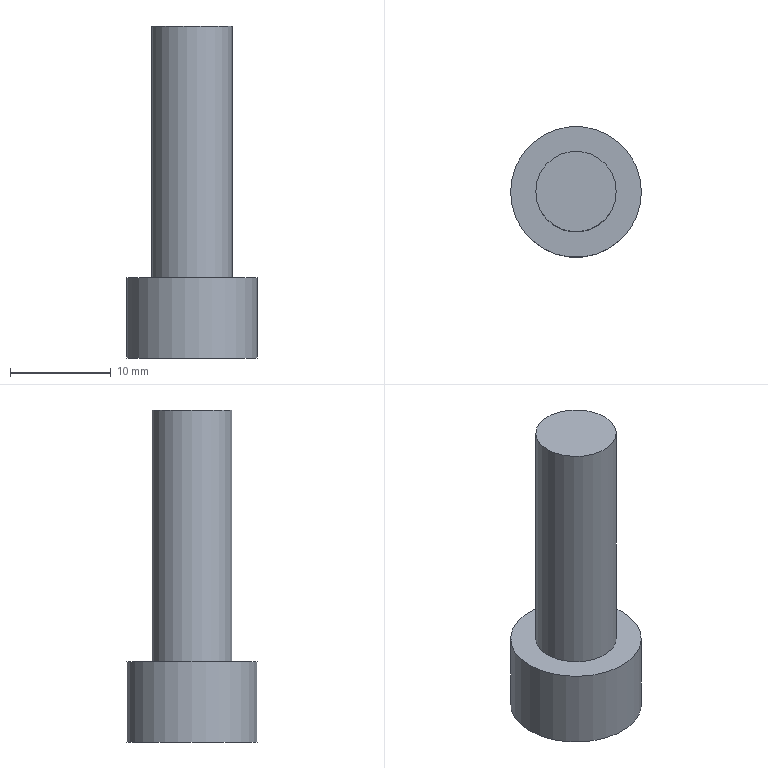Part | STEP file | 1 solid | 12 faces | box 13 x 13 x 33 mm | volume 2154 mm3 | plane 10 | cylinder 2 | commonest cylinder face diameters 8 x1 13 x1
STEP:
#1=CARTESIAN_POINT('',(0.,0.,0.));
#2=DIRECTION('',(0.,0.,1.));
#3=DIRECTION('',(1.,0.,0.));
#4=AXIS2_PLACEMENT_3D('',#1,#2,#3);
#5=CARTESIAN_POINT('',(1550.747,372.48,24.619));
#6=VERTEX_POINT('',#5);
#7=CARTESIAN_POINT('',(1557.247,372.48,24.619));
#8=DIRECTION('',(0.,0.,-1.));
#9=DIRECTION('',(-1.,0.,0.));
#10=AXIS2_PLACEMENT_3D('',#7,#8,#9);
#11=CIRCLE('',#10,6.5);
#12=CARTESIAN_POINT('',(1550.747,372.48,24.619));
#13=DIRECTION('',(0.,0.,1.));
#14=DIRECTION('',(1.,0.,0.));
#15=AXIS2_PLACEMENT_3D('',#12,#13,#14);
#16=PLANE('',#15);
#17=CARTESIAN_POINT('',(0.,0.));
#18=CARTESIAN_POINT('',(0.,11.258));
#19=CARTESIAN_POINT('',(9.75,5.629));
#20=CARTESIAN_POINT('',(19.5,0.));
#21=CARTESIAN_POINT('',(9.75,-5.629));
#22=CARTESIAN_POINT('',(0.,-11.258));
#23=CARTESIAN_POINT('',(0.,0.));
#24=(BOUNDED_CURVE()B_SPLINE_CURVE(2,(#17,#18,#19,#20,#21,#22,#23),.UNSPECIFIED.,.T.,.F.)B_SPLINE_CURVE_WITH_KNOTS((1,2,2,2,2,1),(-2.094,0.,2.094,4.189,6.283,8.378),.UNSPECIFIED.)CURVE()GEOMETRIC_REPRESENTATION_ITEM()RATIONAL_B_SPLINE_CURVE((1.,0.5,1.,0.5,1.,0.5,1.))REPRESENTATION_ITEM(''));
#25=(GEOMETRIC_REPRESENTATION_CONTEXT(2)PARAMETRIC_REPRESENTATION_CONTEXT()REPRESENTATION_CONTEXT('',''));
#26=DEFINITIONAL_REPRESENTATION('',(#24),#25);
#27=PCURVE('',#16,#26);
#28=CARTESIAN_POINT('',(1557.247,372.48,79.519));
#29=DIRECTION('',(0.,0.,-1.));
#30=DIRECTION('',(-1.,0.,0.));
#31=AXIS2_PLACEMENT_3D('',#28,#29,#30);
#32=CYLINDRICAL_SURFACE('',#31,6.5);
#33=CARTESIAN_POINT('',(0.,54.9));
#34=DIRECTION('',(1.,0.));
#35=VECTOR('',#34,1.);
#36=LINE('',#33,#35);
#37=(GEOMETRIC_REPRESENTATION_CONTEXT(2)PARAMETRIC_REPRESENTATION_CONTEXT()REPRESENTATION_CONTEXT('',''));
#38=DEFINITIONAL_REPRESENTATION('',(#36),#37);
#39=PCURVE('',#32,#38);
#40=SURFACE_CURVE('',#11,(#27,#39),.PCURVE_S1.);
#41=EDGE_CURVE('',#6,#6,#40,.T.);
#42=ORIENTED_EDGE('',*,*,#41,.T.);
#43=EDGE_LOOP('',(#42));
#44=FACE_BOUND('',#43,.T.);
#45=CARTESIAN_POINT('',(1558.979,375.48,24.619));
#46=VERTEX_POINT('',#45);
#47=CARTESIAN_POINT('',(1555.515,375.48,24.619));
#48=VERTEX_POINT('',#47);
#49=CARTESIAN_POINT('',(1558.979,375.48,24.619));
#50=DIRECTION('',(-1.,0.,0.));
#51=VECTOR('',#50,1.);
#52=LINE('',#49,#51);
#53=CARTESIAN_POINT('',(8.232,3.));
#54=DIRECTION('',(-1.,0.));
#55=VECTOR('',#54,1.);
#56=LINE('',#53,#55);
#57=(GEOMETRIC_REPRESENTATION_CONTEXT(2)PARAMETRIC_REPRESENTATION_CONTEXT()REPRESENTATION_CONTEXT('',''));
#58=DEFINITIONAL_REPRESENTATION('',(#56),#57);
#59=PCURVE('',#16,#58);
#60=CARTESIAN_POINT('',(1558.979,375.48,29.899));
#61=DIRECTION('',(0.,-1.,0.));
#62=DIRECTION('',(-1.,0.,0.));
#63=AXIS2_PLACEMENT_3D('',#60,#61,#62);
#64=PLANE('',#63);
#65=CARTESIAN_POINT('',(0.,5.28));
#66=DIRECTION('',(1.,0.));
#67=VECTOR('',#66,1.);
#68=LINE('',#65,#67);
#69=(GEOMETRIC_REPRESENTATION_CONTEXT(2)PARAMETRIC_REPRESENTATION_CONTEXT()REPRESENTATION_CONTEXT('',''));
#70=DEFINITIONAL_REPRESENTATION('',(#68),#69);
#71=PCURVE('',#64,#70);
#72=SURFACE_CURVE('',#52,(#59,#71),.PCURVE_S1.);
#73=EDGE_CURVE('',#46,#48,#72,.T.);
#74=ORIENTED_EDGE('',*,*,#73,.T.);
#75=CARTESIAN_POINT('',(1553.783,372.48,24.619));
#76=VERTEX_POINT('',#75);
#77=CARTESIAN_POINT('',(1555.515,375.48,24.619));
#78=DIRECTION('',(-0.5,-0.866,0.));
#79=VECTOR('',#78,1.);
#80=LINE('',#77,#79);
#81=CARTESIAN_POINT('',(4.768,3.));
#82=DIRECTION('',(-0.5,-0.866));
#83=VECTOR('',#82,1.);
#84=LINE('',#81,#83);
#85=(GEOMETRIC_REPRESENTATION_CONTEXT(2)PARAMETRIC_REPRESENTATION_CONTEXT()REPRESENTATION_CONTEXT('',''));
#86=DEFINITIONAL_REPRESENTATION('',(#84),#85);
#87=PCURVE('',#16,#86);
#88=CARTESIAN_POINT('',(1555.515,375.48,29.899));
#89=DIRECTION('',(0.866,-0.5,0.));
#90=DIRECTION('',(-0.5,-0.866,0.));
#91=AXIS2_PLACEMENT_3D('',#88,#89,#90);
#92=PLANE('',#91);
#93=CARTESIAN_POINT('',(0.,5.28));
#94=DIRECTION('',(1.,0.));
#95=VECTOR('',#94,1.);
#96=LINE('',#93,#95);
#97=(GEOMETRIC_REPRESENTATION_CONTEXT(2)PARAMETRIC_REPRESENTATION_CONTEXT()REPRESENTATION_CONTEXT('',''));
#98=DEFINITIONAL_REPRESENTATION('',(#96),#97);
#99=PCURVE('',#92,#98);
#100=SURFACE_CURVE('',#80,(#87,#99),.PCURVE_S1.);
#101=EDGE_CURVE('',#48,#76,#100,.T.);
#102=ORIENTED_EDGE('',*,*,#101,.T.);
#103=CARTESIAN_POINT('',(1555.515,369.48,24.619));
#104=VERTEX_POINT('',#103);
#105=CARTESIAN_POINT('',(1553.783,372.48,24.619));
#106=DIRECTION('',(0.5,-0.866,0.));
#107=VECTOR('',#106,1.);
#108=LINE('',#105,#107);
#109=CARTESIAN_POINT('',(3.036,0.));
#110=DIRECTION('',(0.5,-0.866));
#111=VECTOR('',#110,1.);
#112=LINE('',#109,#111);
#113=(GEOMETRIC_REPRESENTATION_CONTEXT(2)PARAMETRIC_REPRESENTATION_CONTEXT()REPRESENTATION_CONTEXT('',''));
#114=DEFINITIONAL_REPRESENTATION('',(#112),#113);
#115=PCURVE('',#16,#114);
#116=CARTESIAN_POINT('',(1553.783,372.48,29.899));
#117=DIRECTION('',(0.866,0.5,0.));
#118=DIRECTION('',(0.5,-0.866,0.));
#119=AXIS2_PLACEMENT_3D('',#116,#117,#118);
#120=PLANE('',#119);
#121=CARTESIAN_POINT('',(0.,5.28));
#122=DIRECTION('',(1.,0.));
#123=VECTOR('',#122,1.);
#124=LINE('',#121,#123);
#125=(GEOMETRIC_REPRESENTATION_CONTEXT(2)PARAMETRIC_REPRESENTATION_CONTEXT()REPRESENTATION_CONTEXT('',''));
#126=DEFINITIONAL_REPRESENTATION('',(#124),#125);
#127=PCURVE('',#120,#126);
#128=SURFACE_CURVE('',#108,(#115,#127),.PCURVE_S1.);
#129=EDGE_CURVE('',#76,#104,#128,.T.);
#130=ORIENTED_EDGE('',*,*,#129,.T.);
#131=CARTESIAN_POINT('',(1558.979,369.48,24.619));
#132=VERTEX_POINT('',#131);
#133=CARTESIAN_POINT('',(1555.515,369.48,24.619));
#134=DIRECTION('',(1.,0.,0.));
#135=VECTOR('',#134,1.);
#136=LINE('',#133,#135);
#137=CARTESIAN_POINT('',(4.768,-3.));
#138=DIRECTION('',(1.,0.));
#139=VECTOR('',#138,1.);
#140=LINE('',#137,#139);
#141=(GEOMETRIC_REPRESENTATION_CONTEXT(2)PARAMETRIC_REPRESENTATION_CONTEXT()REPRESENTATION_CONTEXT('',''));
#142=DEFINITIONAL_REPRESENTATION('',(#140),#141);
#143=PCURVE('',#16,#142);
#144=CARTESIAN_POINT('',(1555.515,369.48,29.899));
#145=DIRECTION('',(0.,1.,0.));
#146=DIRECTION('',(1.,0.,0.));
#147=AXIS2_PLACEMENT_3D('',#144,#145,#146);
#148=PLANE('',#147);
#149=CARTESIAN_POINT('',(0.,5.28));
#150=DIRECTION('',(1.,0.));
#151=VECTOR('',#150,1.);
#152=LINE('',#149,#151);
#153=(GEOMETRIC_REPRESENTATION_CONTEXT(2)PARAMETRIC_REPRESENTATION_CONTEXT()REPRESENTATION_CONTEXT('',''));
#154=DEFINITIONAL_REPRESENTATION('',(#152),#153);
#155=PCURVE('',#148,#154);
#156=SURFACE_CURVE('',#136,(#143,#155),.PCURVE_S1.);
#157=EDGE_CURVE('',#104,#132,#156,.T.);
#158=ORIENTED_EDGE('',*,*,#157,.T.);
#159=CARTESIAN_POINT('',(1560.711,372.48,24.619));
#160=VERTEX_POINT('',#159);
#161=CARTESIAN_POINT('',(1558.979,369.48,24.619));
#162=DIRECTION('',(0.5,0.866,0.));
#163=VECTOR('',#162,1.);
#164=LINE('',#161,#163);
#165=CARTESIAN_POINT('',(8.232,-3.));
#166=DIRECTION('',(0.5,0.866));
#167=VECTOR('',#166,1.);
#168=LINE('',#165,#167);
#169=(GEOMETRIC_REPRESENTATION_CONTEXT(2)PARAMETRIC_REPRESENTATION_CONTEXT()REPRESENTATION_CONTEXT('',''));
#170=DEFINITIONAL_REPRESENTATION('',(#168),#169);
#171=PCURVE('',#16,#170);
#172=CARTESIAN_POINT('',(1558.979,369.48,29.899));
#173=DIRECTION('',(-0.866,0.5,0.));
#174=DIRECTION('',(0.5,0.866,0.));
#175=AXIS2_PLACEMENT_3D('',#172,#173,#174);
#176=PLANE('',#175);
#177=CARTESIAN_POINT('',(0.,5.28));
#178=DIRECTION('',(1.,0.));
#179=VECTOR('',#178,1.);
#180=LINE('',#177,#179);
#181=(GEOMETRIC_REPRESENTATION_CONTEXT(2)PARAMETRIC_REPRESENTATION_CONTEXT()REPRESENTATION_CONTEXT('',''));
#182=DEFINITIONAL_REPRESENTATION('',(#180),#181);
#183=PCURVE('',#176,#182);
#184=SURFACE_CURVE('',#164,(#171,#183),.PCURVE_S1.);
#185=EDGE_CURVE('',#132,#160,#184,.T.);
#186=ORIENTED_EDGE('',*,*,#185,.T.);
#187=CARTESIAN_POINT('',(1560.711,372.48,24.619));
#188=DIRECTION('',(-0.5,0.866,0.));
#189=VECTOR('',#188,1.);
#190=LINE('',#187,#189);
#191=CARTESIAN_POINT('',(9.964,0.));
#192=DIRECTION('',(-0.5,0.866));
#193=VECTOR('',#192,1.);
#194=LINE('',#191,#193);
#195=(GEOMETRIC_REPRESENTATION_CONTEXT(2)PARAMETRIC_REPRESENTATION_CONTEXT()REPRESENTATION_CONTEXT('',''));
#196=DEFINITIONAL_REPRESENTATION('',(#194),#195);
#197=PCURVE('',#16,#196);
#198=CARTESIAN_POINT('',(1560.711,372.48,29.899));
#199=DIRECTION('',(-0.866,-0.5,0.));
#200=DIRECTION('',(-0.5,0.866,0.));
#201=AXIS2_PLACEMENT_3D('',#198,#199,#200);
#202=PLANE('',#201);
#203=CARTESIAN_POINT('',(0.,5.28));
#204=DIRECTION('',(1.,0.));
#205=VECTOR('',#204,1.);
#206=LINE('',#203,#205);
#207=(GEOMETRIC_REPRESENTATION_CONTEXT(2)PARAMETRIC_REPRESENTATION_CONTEXT()REPRESENTATION_CONTEXT('',''));
#208=DEFINITIONAL_REPRESENTATION('',(#206),#207);
#209=PCURVE('',#202,#208);
#210=SURFACE_CURVE('',#190,(#197,#209),.PCURVE_S1.);
#211=EDGE_CURVE('',#160,#46,#210,.T.);
#212=ORIENTED_EDGE('',*,*,#211,.T.);
#213=EDGE_LOOP('',(#74,#102,#130,#158,#186,#212));
#214=FACE_BOUND('',#213,.T.);
#215=ADVANCED_FACE('',(#44,#214),#16,.F.);
#216=ORIENTED_EDGE('',*,*,#41,.F.);
#217=CARTESIAN_POINT('',(1550.747,372.48,32.619));
#218=VERTEX_POINT('',#217);
#219=CARTESIAN_POINT('',(1550.747,372.48,32.619));
#220=CARTESIAN_POINT('',(1550.747,372.48,24.619));
#221=B_SPLINE_CURVE_WITH_KNOTS('',1,(#219,#220),.UNSPECIFIED.,.F.,.F.,(2,2),(46.9,54.9),.PIECEWISE_BEZIER_KNOTS.);
#222=CARTESIAN_POINT('',(0.,0.));
#223=DIRECTION('',(0.,1.));
#224=VECTOR('',#223,1.);
#225=LINE('',#222,#224);
#226=(GEOMETRIC_REPRESENTATION_CONTEXT(2)PARAMETRIC_REPRESENTATION_CONTEXT()REPRESENTATION_CONTEXT('',''));
#227=DEFINITIONAL_REPRESENTATION('',(#225),#226);
#228=PCURVE('',#32,#227);
#229=CARTESIAN_POINT('',(6.283,0.));
#230=DIRECTION('',(0.,1.));
#231=VECTOR('',#230,1.);
#232=LINE('',#229,#231);
#233=(GEOMETRIC_REPRESENTATION_CONTEXT(2)PARAMETRIC_REPRESENTATION_CONTEXT()REPRESENTATION_CONTEXT('',''));
#234=DEFINITIONAL_REPRESENTATION('',(#232),#233);
#235=PCURVE('',#32,#234);
#236=SEAM_CURVE('',#221,(#228,#235),.PCURVE_S1.);
#237=EDGE_CURVE('',#218,#6,#236,.T.);
#238=ORIENTED_EDGE('',*,*,#237,.F.);
#239=CARTESIAN_POINT('',(1557.247,372.48,32.619));
#240=DIRECTION('',(0.,0.,-1.));
#241=DIRECTION('',(-1.,0.,0.));
#242=AXIS2_PLACEMENT_3D('',#239,#240,#241);
#243=CIRCLE('',#242,6.5);
#244=CARTESIAN_POINT('',(0.,46.9));
#245=DIRECTION('',(1.,0.));
#246=VECTOR('',#245,1.);
#247=LINE('',#244,#246);
#248=(GEOMETRIC_REPRESENTATION_CONTEXT(2)PARAMETRIC_REPRESENTATION_CONTEXT()REPRESENTATION_CONTEXT('',''));
#249=DEFINITIONAL_REPRESENTATION('',(#247),#248);
#250=PCURVE('',#32,#249);
#251=CARTESIAN_POINT('',(1553.247,372.48,32.619));
#252=DIRECTION('',(0.,0.,-1.));
#253=DIRECTION('',(-1.,0.,0.));
#254=AXIS2_PLACEMENT_3D('',#251,#252,#253);
#255=PLANE('',#254);
#256=CARTESIAN_POINT('',(-4.,0.));
#257=DIRECTION('',(1.,0.));
#258=AXIS2_PLACEMENT_2D('',#256,#257);
#259=CIRCLE('',#258,6.5);
#260=(GEOMETRIC_REPRESENTATION_CONTEXT(2)PARAMETRIC_REPRESENTATION_CONTEXT()REPRESENTATION_CONTEXT('',''));
#261=DEFINITIONAL_REPRESENTATION('',(#259),#260);
#262=PCURVE('',#255,#261);
#263=SURFACE_CURVE('',#243,(#250,#262),.PCURVE_S1.);
#264=EDGE_CURVE('',#218,#218,#263,.T.);
#265=ORIENTED_EDGE('',*,*,#264,.T.);
#266=ORIENTED_EDGE('',*,*,#237,.T.);
#267=EDGE_LOOP('',(#216,#238,#265,#266));
#268=FACE_BOUND('',#267,.T.);
#269=ADVANCED_FACE('',(#268),#32,.T.);
#270=ORIENTED_EDGE('',*,*,#264,.F.);
#271=EDGE_LOOP('',(#270));
#272=FACE_BOUND('',#271,.T.);
#273=CARTESIAN_POINT('',(1553.247,372.48,32.619));
#274=VERTEX_POINT('',#273);
#275=CARTESIAN_POINT('',(1557.247,372.48,32.619));
#276=DIRECTION('',(0.,0.,-1.));
#277=DIRECTION('',(-1.,0.,0.));
#278=AXIS2_PLACEMENT_3D('',#275,#276,#277);
#279=CIRCLE('',#278,4.);
#280=CARTESIAN_POINT('',(-4.,0.));
#281=DIRECTION('',(1.,0.));
#282=AXIS2_PLACEMENT_2D('',#280,#281);
#283=CIRCLE('',#282,4.);
#284=(GEOMETRIC_REPRESENTATION_CONTEXT(2)PARAMETRIC_REPRESENTATION_CONTEXT()REPRESENTATION_CONTEXT('',''));
#285=DEFINITIONAL_REPRESENTATION('',(#283),#284);
#286=PCURVE('',#255,#285);
#287=CARTESIAN_POINT('',(1557.247,372.48,79.519));
#288=DIRECTION('',(0.,0.,-1.));
#289=DIRECTION('',(-1.,0.,0.));
#290=AXIS2_PLACEMENT_3D('',#287,#288,#289);
#291=CYLINDRICAL_SURFACE('',#290,4.);
#292=CARTESIAN_POINT('',(0.,46.9));
#293=DIRECTION('',(1.,0.));
#294=VECTOR('',#293,1.);
#295=LINE('',#292,#294);
#296=(GEOMETRIC_REPRESENTATION_CONTEXT(2)PARAMETRIC_REPRESENTATION_CONTEXT()REPRESENTATION_CONTEXT('',''));
#297=DEFINITIONAL_REPRESENTATION('',(#295),#296);
#298=PCURVE('',#291,#297);
#299=SURFACE_CURVE('',#279,(#286,#298),.PCURVE_S1.);
#300=EDGE_CURVE('',#274,#274,#299,.T.);
#301=ORIENTED_EDGE('',*,*,#300,.T.);
#302=EDGE_LOOP('',(#301));
#303=FACE_BOUND('',#302,.T.);
#304=ADVANCED_FACE('',(#272,#303),#255,.F.);
#305=ORIENTED_EDGE('',*,*,#300,.F.);
#306=CARTESIAN_POINT('',(1553.247,372.48,57.619));
#307=VERTEX_POINT('',#306);
#308=CARTESIAN_POINT('',(1553.247,372.48,57.619));
#309=CARTESIAN_POINT('',(1553.247,372.48,32.619));
#310=B_SPLINE_CURVE_WITH_KNOTS('',1,(#308,#309),.UNSPECIFIED.,.F.,.F.,(2,2),(21.9,46.9),.PIECEWISE_BEZIER_KNOTS.);
#311=CARTESIAN_POINT('',(0.,0.));
#312=DIRECTION('',(0.,1.));
#313=VECTOR('',#312,1.);
#314=LINE('',#311,#313);
#315=(GEOMETRIC_REPRESENTATION_CONTEXT(2)PARAMETRIC_REPRESENTATION_CONTEXT()REPRESENTATION_CONTEXT('',''));
#316=DEFINITIONAL_REPRESENTATION('',(#314),#315);
#317=PCURVE('',#291,#316);
#318=CARTESIAN_POINT('',(6.283,0.));
#319=DIRECTION('',(0.,1.));
#320=VECTOR('',#319,1.);
#321=LINE('',#318,#320);
#322=(GEOMETRIC_REPRESENTATION_CONTEXT(2)PARAMETRIC_REPRESENTATION_CONTEXT()REPRESENTATION_CONTEXT('',''));
#323=DEFINITIONAL_REPRESENTATION('',(#321),#322);
#324=PCURVE('',#291,#323);
#325=SEAM_CURVE('',#310,(#317,#324),.PCURVE_S1.);
#326=EDGE_CURVE('',#307,#274,#325,.T.);
#327=ORIENTED_EDGE('',*,*,#326,.F.);
#328=CARTESIAN_POINT('',(1557.247,372.48,57.619));
#329=DIRECTION('',(0.,0.,-1.));
#330=DIRECTION('',(-1.,0.,0.));
#331=AXIS2_PLACEMENT_3D('',#328,#329,#330);
#332=CIRCLE('',#331,4.);
#333=CARTESIAN_POINT('',(0.,21.9));
#334=DIRECTION('',(1.,0.));
#335=VECTOR('',#334,1.);
#336=LINE('',#333,#335);
#337=(GEOMETRIC_REPRESENTATION_CONTEXT(2)PARAMETRIC_REPRESENTATION_CONTEXT()REPRESENTATION_CONTEXT('',''));
#338=DEFINITIONAL_REPRESENTATION('',(#336),#337);
#339=PCURVE('',#291,#338);
#340=CARTESIAN_POINT('',(1557.247,372.48,57.619));
#341=DIRECTION('',(0.,0.,-1.));
#342=DIRECTION('',(-1.,0.,0.));
#343=AXIS2_PLACEMENT_3D('',#340,#341,#342);
#344=PLANE('',#343);
#345=CARTESIAN_POINT('',(0.,0.));
#346=DIRECTION('',(1.,0.));
#347=AXIS2_PLACEMENT_2D('',#345,#346);
#348=CIRCLE('',#347,4.);
#349=(GEOMETRIC_REPRESENTATION_CONTEXT(2)PARAMETRIC_REPRESENTATION_CONTEXT()REPRESENTATION_CONTEXT('',''));
#350=DEFINITIONAL_REPRESENTATION('',(#348),#349);
#351=PCURVE('',#344,#350);
#352=SURFACE_CURVE('',#332,(#339,#351),.PCURVE_S1.);
#353=EDGE_CURVE('',#307,#307,#352,.T.);
#354=ORIENTED_EDGE('',*,*,#353,.T.);
#355=ORIENTED_EDGE('',*,*,#326,.T.);
#356=EDGE_LOOP('',(#305,#327,#354,#355));
#357=FACE_BOUND('',#356,.T.);
#358=ADVANCED_FACE('',(#357),#291,.T.);
#359=ORIENTED_EDGE('',*,*,#353,.F.);
#360=EDGE_LOOP('',(#359));
#361=FACE_BOUND('',#360,.T.);
#362=ADVANCED_FACE('',(#361),#344,.F.);
#363=ORIENTED_EDGE('',*,*,#73,.F.);
#364=CARTESIAN_POINT('',(1558.979,375.48,29.899));
#365=VERTEX_POINT('',#364);
#366=CARTESIAN_POINT('',(1558.979,375.48,29.899));
#367=DIRECTION('',(0.,0.,1.));
#368=VECTOR('',#367,1.);
#369=LINE('',#366,#368);
#370=CARTESIAN_POINT('',(0.,0.));
#371=DIRECTION('',(0.,-1.));
#372=VECTOR('',#371,1.);
#373=LINE('',#370,#372);
#374=(GEOMETRIC_REPRESENTATION_CONTEXT(2)PARAMETRIC_REPRESENTATION_CONTEXT()REPRESENTATION_CONTEXT('',''));
#375=DEFINITIONAL_REPRESENTATION('',(#373),#374);
#376=PCURVE('',#64,#375);
#377=CARTESIAN_POINT('',(3.464,0.));
#378=DIRECTION('',(0.,-1.));
#379=VECTOR('',#378,1.);
#380=LINE('',#377,#379);
#381=(GEOMETRIC_REPRESENTATION_CONTEXT(2)PARAMETRIC_REPRESENTATION_CONTEXT()REPRESENTATION_CONTEXT('',''));
#382=DEFINITIONAL_REPRESENTATION('',(#380),#381);
#383=PCURVE('',#202,#382);
#384=SURFACE_CURVE('',#369,(#376,#383),.PCURVE_S1.);
#385=EDGE_CURVE('',#46,#365,#384,.T.);
#386=ORIENTED_EDGE('',*,*,#385,.T.);
#387=CARTESIAN_POINT('',(1555.515,375.48,29.899));
#388=VERTEX_POINT('',#387);
#389=CARTESIAN_POINT('',(1558.979,375.48,29.899));
#390=DIRECTION('',(1.,0.,0.));
#391=VECTOR('',#390,1.);
#392=LINE('',#389,#391);
#393=CARTESIAN_POINT('',(0.,0.));
#394=DIRECTION('',(-1.,0.));
#395=VECTOR('',#394,1.);
#396=LINE('',#393,#395);
#397=(GEOMETRIC_REPRESENTATION_CONTEXT(2)PARAMETRIC_REPRESENTATION_CONTEXT()REPRESENTATION_CONTEXT('',''));
#398=DEFINITIONAL_REPRESENTATION('',(#396),#397);
#399=PCURVE('',#64,#398);
#400=CARTESIAN_POINT('',(1557.247,372.48,29.899));
#401=DIRECTION('',(0.,0.,1.));
#402=DIRECTION('',(1.,0.,0.));
#403=AXIS2_PLACEMENT_3D('',#400,#401,#402);
#404=PLANE('',#403);
#405=CARTESIAN_POINT('',(1.732,3.));
#406=DIRECTION('',(1.,0.));
#407=VECTOR('',#406,1.);
#408=LINE('',#405,#407);
#409=(GEOMETRIC_REPRESENTATION_CONTEXT(2)PARAMETRIC_REPRESENTATION_CONTEXT()REPRESENTATION_CONTEXT('',''));
#410=DEFINITIONAL_REPRESENTATION('',(#408),#409);
#411=PCURVE('',#404,#410);
#412=SURFACE_CURVE('',#392,(#399,#411),.PCURVE_S1.);
#413=EDGE_CURVE('',#388,#365,#412,.T.);
#414=ORIENTED_EDGE('',*,*,#413,.F.);
#415=CARTESIAN_POINT('',(1555.515,375.48,29.899));
#416=DIRECTION('',(0.,0.,1.));
#417=VECTOR('',#416,1.);
#418=LINE('',#415,#417);
#419=CARTESIAN_POINT('',(3.464,0.));
#420=DIRECTION('',(0.,-1.));
#421=VECTOR('',#420,1.);
#422=LINE('',#419,#421);
#423=(GEOMETRIC_REPRESENTATION_CONTEXT(2)PARAMETRIC_REPRESENTATION_CONTEXT()REPRESENTATION_CONTEXT('',''));
#424=DEFINITIONAL_REPRESENTATION('',(#422),#423);
#425=PCURVE('',#64,#424);
#426=CARTESIAN_POINT('',(0.,0.));
#427=DIRECTION('',(0.,-1.));
#428=VECTOR('',#427,1.);
#429=LINE('',#426,#428);
#430=(GEOMETRIC_REPRESENTATION_CONTEXT(2)PARAMETRIC_REPRESENTATION_CONTEXT()REPRESENTATION_CONTEXT('',''));
#431=DEFINITIONAL_REPRESENTATION('',(#429),#430);
#432=PCURVE('',#92,#431);
#433=SURFACE_CURVE('',#418,(#425,#432),.PCURVE_S1.);
#434=EDGE_CURVE('',#48,#388,#433,.T.);
#435=ORIENTED_EDGE('',*,*,#434,.F.);
#436=EDGE_LOOP('',(#363,#386,#414,#435));
#437=FACE_BOUND('',#436,.T.);
#438=ADVANCED_FACE('',(#437),#64,.T.);
#439=ORIENTED_EDGE('',*,*,#101,.F.);
#440=ORIENTED_EDGE('',*,*,#434,.T.);
#441=CARTESIAN_POINT('',(1553.783,372.48,29.899));
#442=VERTEX_POINT('',#441);
#443=CARTESIAN_POINT('',(1555.515,375.48,29.899));
#444=DIRECTION('',(0.5,0.866,0.));
#445=VECTOR('',#444,1.);
#446=LINE('',#443,#445);
#447=CARTESIAN_POINT('',(0.,0.));
#448=DIRECTION('',(-1.,0.));
#449=VECTOR('',#448,1.);
#450=LINE('',#447,#449);
#451=(GEOMETRIC_REPRESENTATION_CONTEXT(2)PARAMETRIC_REPRESENTATION_CONTEXT()REPRESENTATION_CONTEXT('',''));
#452=DEFINITIONAL_REPRESENTATION('',(#450),#451);
#453=PCURVE('',#92,#452);
#454=CARTESIAN_POINT('',(-1.732,3.));
#455=DIRECTION('',(0.5,0.866));
#456=VECTOR('',#455,1.);
#457=LINE('',#454,#456);
#458=(GEOMETRIC_REPRESENTATION_CONTEXT(2)PARAMETRIC_REPRESENTATION_CONTEXT()REPRESENTATION_CONTEXT('',''));
#459=DEFINITIONAL_REPRESENTATION('',(#457),#458);
#460=PCURVE('',#404,#459);
#461=SURFACE_CURVE('',#446,(#453,#460),.PCURVE_S1.);
#462=EDGE_CURVE('',#442,#388,#461,.T.);
#463=ORIENTED_EDGE('',*,*,#462,.F.);
#464=CARTESIAN_POINT('',(1553.783,372.48,29.899));
#465=DIRECTION('',(0.,0.,1.));
#466=VECTOR('',#465,1.);
#467=LINE('',#464,#466);
#468=CARTESIAN_POINT('',(3.464,0.));
#469=DIRECTION('',(0.,-1.));
#470=VECTOR('',#469,1.);
#471=LINE('',#468,#470);
#472=(GEOMETRIC_REPRESENTATION_CONTEXT(2)PARAMETRIC_REPRESENTATION_CONTEXT()REPRESENTATION_CONTEXT('',''));
#473=DEFINITIONAL_REPRESENTATION('',(#471),#472);
#474=PCURVE('',#92,#473);
#475=CARTESIAN_POINT('',(0.,0.));
#476=DIRECTION('',(0.,-1.));
#477=VECTOR('',#476,1.);
#478=LINE('',#475,#477);
#479=(GEOMETRIC_REPRESENTATION_CONTEXT(2)PARAMETRIC_REPRESENTATION_CONTEXT()REPRESENTATION_CONTEXT('',''));
#480=DEFINITIONAL_REPRESENTATION('',(#478),#479);
#481=PCURVE('',#120,#480);
#482=SURFACE_CURVE('',#467,(#474,#481),.PCURVE_S1.);
#483=EDGE_CURVE('',#76,#442,#482,.T.);
#484=ORIENTED_EDGE('',*,*,#483,.F.);
#485=EDGE_LOOP('',(#439,#440,#463,#484));
#486=FACE_BOUND('',#485,.T.);
#487=ADVANCED_FACE('',(#486),#92,.T.);
#488=ORIENTED_EDGE('',*,*,#129,.F.);
#489=ORIENTED_EDGE('',*,*,#483,.T.);
#490=CARTESIAN_POINT('',(1555.515,369.48,29.899));
#491=VERTEX_POINT('',#490);
#492=CARTESIAN_POINT('',(1553.783,372.48,29.899));
#493=DIRECTION('',(-0.5,0.866,0.));
#494=VECTOR('',#493,1.);
#495=LINE('',#492,#494);
#496=CARTESIAN_POINT('',(0.,0.));
#497=DIRECTION('',(-1.,0.));
#498=VECTOR('',#497,1.);
#499=LINE('',#496,#498);
#500=(GEOMETRIC_REPRESENTATION_CONTEXT(2)PARAMETRIC_REPRESENTATION_CONTEXT()REPRESENTATION_CONTEXT('',''));
#501=DEFINITIONAL_REPRESENTATION('',(#499),#500);
#502=PCURVE('',#120,#501);
#503=CARTESIAN_POINT('',(-3.464,0.));
#504=DIRECTION('',(-0.5,0.866));
#505=VECTOR('',#504,1.);
#506=LINE('',#503,#505);
#507=(GEOMETRIC_REPRESENTATION_CONTEXT(2)PARAMETRIC_REPRESENTATION_CONTEXT()REPRESENTATION_CONTEXT('',''));
#508=DEFINITIONAL_REPRESENTATION('',(#506),#507);
#509=PCURVE('',#404,#508);
#510=SURFACE_CURVE('',#495,(#502,#509),.PCURVE_S1.);
#511=EDGE_CURVE('',#491,#442,#510,.T.);
#512=ORIENTED_EDGE('',*,*,#511,.F.);
#513=CARTESIAN_POINT('',(1555.515,369.48,29.899));
#514=DIRECTION('',(0.,0.,1.));
#515=VECTOR('',#514,1.);
#516=LINE('',#513,#515);
#517=CARTESIAN_POINT('',(3.464,0.));
#518=DIRECTION('',(0.,-1.));
#519=VECTOR('',#518,1.);
#520=LINE('',#517,#519);
#521=(GEOMETRIC_REPRESENTATION_CONTEXT(2)PARAMETRIC_REPRESENTATION_CONTEXT()REPRESENTATION_CONTEXT('',''));
#522=DEFINITIONAL_REPRESENTATION('',(#520),#521);
#523=PCURVE('',#120,#522);
#524=CARTESIAN_POINT('',(0.,0.));
#525=DIRECTION('',(0.,-1.));
#526=VECTOR('',#525,1.);
#527=LINE('',#524,#526);
#528=(GEOMETRIC_REPRESENTATION_CONTEXT(2)PARAMETRIC_REPRESENTATION_CONTEXT()REPRESENTATION_CONTEXT('',''));
#529=DEFINITIONAL_REPRESENTATION('',(#527),#528);
#530=PCURVE('',#148,#529);
#531=SURFACE_CURVE('',#516,(#523,#530),.PCURVE_S1.);
#532=EDGE_CURVE('',#104,#491,#531,.T.);
#533=ORIENTED_EDGE('',*,*,#532,.F.);
#534=EDGE_LOOP('',(#488,#489,#512,#533));
#535=FACE_BOUND('',#534,.T.);
#536=ADVANCED_FACE('',(#535),#120,.T.);
#537=ORIENTED_EDGE('',*,*,#157,.F.);
#538=ORIENTED_EDGE('',*,*,#532,.T.);
#539=CARTESIAN_POINT('',(1558.979,369.48,29.899));
#540=VERTEX_POINT('',#539);
#541=CARTESIAN_POINT('',(1555.515,369.48,29.899));
#542=DIRECTION('',(-1.,0.,0.));
#543=VECTOR('',#542,1.);
#544=LINE('',#541,#543);
#545=CARTESIAN_POINT('',(0.,0.));
#546=DIRECTION('',(-1.,0.));
#547=VECTOR('',#546,1.);
#548=LINE('',#545,#547);
#549=(GEOMETRIC_REPRESENTATION_CONTEXT(2)PARAMETRIC_REPRESENTATION_CONTEXT()REPRESENTATION_CONTEXT('',''));
#550=DEFINITIONAL_REPRESENTATION('',(#548),#549);
#551=PCURVE('',#148,#550);
#552=CARTESIAN_POINT('',(-1.732,-3.));
#553=DIRECTION('',(-1.,0.));
#554=VECTOR('',#553,1.);
#555=LINE('',#552,#554);
#556=(GEOMETRIC_REPRESENTATION_CONTEXT(2)PARAMETRIC_REPRESENTATION_CONTEXT()REPRESENTATION_CONTEXT('',''));
#557=DEFINITIONAL_REPRESENTATION('',(#555),#556);
#558=PCURVE('',#404,#557);
#559=SURFACE_CURVE('',#544,(#551,#558),.PCURVE_S1.);
#560=EDGE_CURVE('',#540,#491,#559,.T.);
#561=ORIENTED_EDGE('',*,*,#560,.F.);
#562=CARTESIAN_POINT('',(1558.979,369.48,29.899));
#563=DIRECTION('',(0.,0.,1.));
#564=VECTOR('',#563,1.);
#565=LINE('',#562,#564);
#566=CARTESIAN_POINT('',(3.464,0.));
#567=DIRECTION('',(0.,-1.));
#568=VECTOR('',#567,1.);
#569=LINE('',#566,#568);
#570=(GEOMETRIC_REPRESENTATION_CONTEXT(2)PARAMETRIC_REPRESENTATION_CONTEXT()REPRESENTATION_CONTEXT('',''));
#571=DEFINITIONAL_REPRESENTATION('',(#569),#570);
#572=PCURVE('',#148,#571);
#573=CARTESIAN_POINT('',(0.,0.));
#574=DIRECTION('',(0.,-1.));
#575=VECTOR('',#574,1.);
#576=LINE('',#573,#575);
#577=(GEOMETRIC_REPRESENTATION_CONTEXT(2)PARAMETRIC_REPRESENTATION_CONTEXT()REPRESENTATION_CONTEXT('',''));
#578=DEFINITIONAL_REPRESENTATION('',(#576),#577);
#579=PCURVE('',#176,#578);
#580=SURFACE_CURVE('',#565,(#572,#579),.PCURVE_S1.);
#581=EDGE_CURVE('',#132,#540,#580,.T.);
#582=ORIENTED_EDGE('',*,*,#581,.F.);
#583=EDGE_LOOP('',(#537,#538,#561,#582));
#584=FACE_BOUND('',#583,.T.);
#585=ADVANCED_FACE('',(#584),#148,.T.);
#586=ORIENTED_EDGE('',*,*,#185,.F.);
#587=ORIENTED_EDGE('',*,*,#581,.T.);
#588=CARTESIAN_POINT('',(1560.711,372.48,29.899));
#589=VERTEX_POINT('',#588);
#590=CARTESIAN_POINT('',(1558.979,369.48,29.899));
#591=DIRECTION('',(-0.5,-0.866,0.));
#592=VECTOR('',#591,1.);
#593=LINE('',#590,#592);
#594=CARTESIAN_POINT('',(0.,0.));
#595=DIRECTION('',(-1.,0.));
#596=VECTOR('',#595,1.);
#597=LINE('',#594,#596);
#598=(GEOMETRIC_REPRESENTATION_CONTEXT(2)PARAMETRIC_REPRESENTATION_CONTEXT()REPRESENTATION_CONTEXT('',''));
#599=DEFINITIONAL_REPRESENTATION('',(#597),#598);
#600=PCURVE('',#176,#599);
#601=CARTESIAN_POINT('',(1.732,-3.));
#602=DIRECTION('',(-0.5,-0.866));
#603=VECTOR('',#602,1.);
#604=LINE('',#601,#603);
#605=(GEOMETRIC_REPRESENTATION_CONTEXT(2)PARAMETRIC_REPRESENTATION_CONTEXT()REPRESENTATION_CONTEXT('',''));
#606=DEFINITIONAL_REPRESENTATION('',(#604),#605);
#607=PCURVE('',#404,#606);
#608=SURFACE_CURVE('',#593,(#600,#607),.PCURVE_S1.);
#609=EDGE_CURVE('',#589,#540,#608,.T.);
#610=ORIENTED_EDGE('',*,*,#609,.F.);
#611=CARTESIAN_POINT('',(1560.711,372.48,29.899));
#612=DIRECTION('',(0.,0.,1.));
#613=VECTOR('',#612,1.);
#614=LINE('',#611,#613);
#615=CARTESIAN_POINT('',(3.464,0.));
#616=DIRECTION('',(0.,-1.));
#617=VECTOR('',#616,1.);
#618=LINE('',#615,#617);
#619=(GEOMETRIC_REPRESENTATION_CONTEXT(2)PARAMETRIC_REPRESENTATION_CONTEXT()REPRESENTATION_CONTEXT('',''));
#620=DEFINITIONAL_REPRESENTATION('',(#618),#619);
#621=PCURVE('',#176,#620);
#622=CARTESIAN_POINT('',(0.,0.));
#623=DIRECTION('',(0.,-1.));
#624=VECTOR('',#623,1.);
#625=LINE('',#622,#624);
#626=(GEOMETRIC_REPRESENTATION_CONTEXT(2)PARAMETRIC_REPRESENTATION_CONTEXT()REPRESENTATION_CONTEXT('',''));
#627=DEFINITIONAL_REPRESENTATION('',(#625),#626);
#628=PCURVE('',#202,#627);
#629=SURFACE_CURVE('',#614,(#621,#628),.PCURVE_S1.);
#630=EDGE_CURVE('',#160,#589,#629,.T.);
#631=ORIENTED_EDGE('',*,*,#630,.F.);
#632=EDGE_LOOP('',(#586,#587,#610,#631));
#633=FACE_BOUND('',#632,.T.);
#634=ADVANCED_FACE('',(#633),#176,.T.);
#635=ORIENTED_EDGE('',*,*,#211,.F.);
#636=ORIENTED_EDGE('',*,*,#630,.T.);
#637=CARTESIAN_POINT('',(1560.711,372.48,29.899));
#638=DIRECTION('',(0.5,-0.866,0.));
#639=VECTOR('',#638,1.);
#640=LINE('',#637,#639);
#641=CARTESIAN_POINT('',(0.,0.));
#642=DIRECTION('',(-1.,0.));
#643=VECTOR('',#642,1.);
#644=LINE('',#641,#643);
#645=(GEOMETRIC_REPRESENTATION_CONTEXT(2)PARAMETRIC_REPRESENTATION_CONTEXT()REPRESENTATION_CONTEXT('',''));
#646=DEFINITIONAL_REPRESENTATION('',(#644),#645);
#647=PCURVE('',#202,#646);
#648=CARTESIAN_POINT('',(3.464,0.));
#649=DIRECTION('',(0.5,-0.866));
#650=VECTOR('',#649,1.);
#651=LINE('',#648,#650);
#652=(GEOMETRIC_REPRESENTATION_CONTEXT(2)PARAMETRIC_REPRESENTATION_CONTEXT()REPRESENTATION_CONTEXT('',''));
#653=DEFINITIONAL_REPRESENTATION('',(#651),#652);
#654=PCURVE('',#404,#653);
#655=SURFACE_CURVE('',#640,(#647,#654),.PCURVE_S1.);
#656=EDGE_CURVE('',#365,#589,#655,.T.);
#657=ORIENTED_EDGE('',*,*,#656,.F.);
#658=ORIENTED_EDGE('',*,*,#385,.F.);
#659=EDGE_LOOP('',(#635,#636,#657,#658));
#660=FACE_BOUND('',#659,.T.);
#661=ADVANCED_FACE('',(#660),#202,.T.);
#662=ORIENTED_EDGE('',*,*,#413,.T.);
#663=ORIENTED_EDGE('',*,*,#656,.T.);
#664=ORIENTED_EDGE('',*,*,#609,.T.);
#665=ORIENTED_EDGE('',*,*,#560,.T.);
#666=ORIENTED_EDGE('',*,*,#511,.T.);
#667=ORIENTED_EDGE('',*,*,#462,.T.);
#668=EDGE_LOOP('',(#662,#663,#664,#665,#666,#667));
#669=FACE_BOUND('',#668,.T.);
#670=ADVANCED_FACE('',(#669),#404,.F.);
#671=CLOSED_SHELL('',(#215,#269,#304,#358,#362,#438,#487,#536,#585,#634,#661,#670));
#672=MANIFOLD_SOLID_BREP('',#671);
#673=(LENGTH_UNIT()NAMED_UNIT(*)SI_UNIT(.MILLI.,.METRE.));
#674=UNCERTAINTY_MEASURE_WITH_UNIT(LENGTH_MEASURE(0.000002),#673,'','');
#675=(NAMED_UNIT(*)PLANE_ANGLE_UNIT()SI_UNIT($,.RADIAN.));
#676=(NAMED_UNIT(*)SI_UNIT($,.STERADIAN.)SOLID_ANGLE_UNIT());
#677=(GEOMETRIC_REPRESENTATION_CONTEXT(3)GLOBAL_UNCERTAINTY_ASSIGNED_CONTEXT((#674))GLOBAL_UNIT_ASSIGNED_CONTEXT((#673,#675,#676))REPRESENTATION_CONTEXT('',''));
#678=ADVANCED_BREP_SHAPE_REPRESENTATION('',(#4,#672),#677);